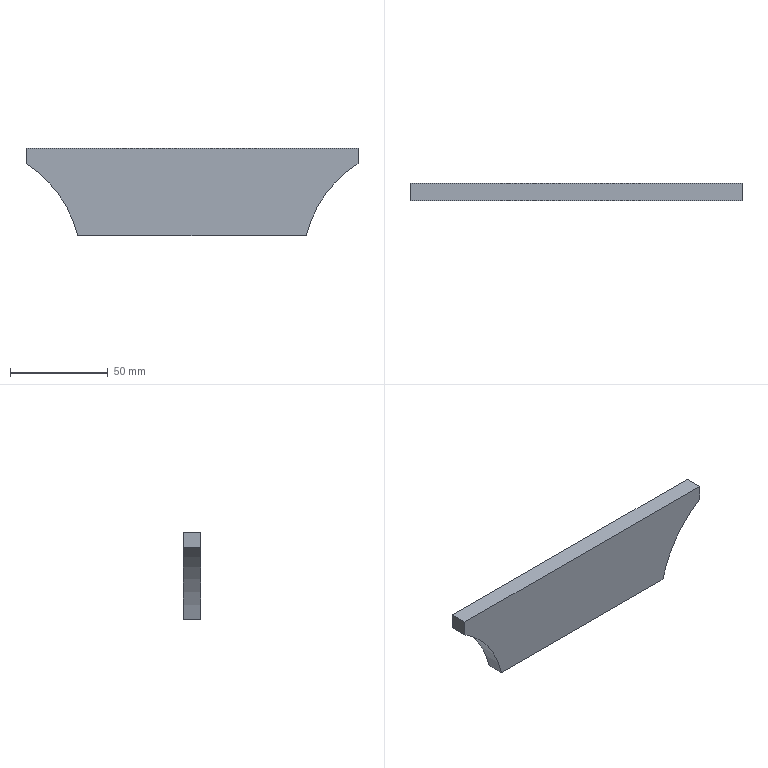Part | SolidWorks | features FlatPattern 1, SMBaseFlange 1, SheetMetal 1 | 1 solid | 8 faces | box 170 x 9 x 45 mm | volume 57559 mm3 | plane 6 | cylinder 2 | commonest cylinder face diameters 120 x2
STEP:
#1=CARTESIAN_POINT('',(0.,0.,-8.));
#2=VERTEX_POINT('',#1);
#3=CARTESIAN_POINT('',(0.,0.,0.));
#4=VERTEX_POINT('',#3);
#5=CARTESIAN_POINT('',(0.,0.,0.));
#6=DIRECTION('',(0.,0.,1.));
#7=VECTOR('',#6,1000.);
#8=LINE('',#5,#7);
#9=EDGE_CURVE('',#2,#4,#8,.T.);
#10=ORIENTED_EDGE('',*,*,#9,.F.);
#11=CARTESIAN_POINT('',(0.,-9.,-8.));
#12=VERTEX_POINT('',#11);
#13=CARTESIAN_POINT('',(0.,-9.,-8.));
#14=DIRECTION('',(0.,1.,0.));
#15=VECTOR('',#14,1000.);
#16=LINE('',#13,#15);
#17=EDGE_CURVE('',#12,#2,#16,.T.);
#18=ORIENTED_EDGE('',*,*,#17,.F.);
#19=CARTESIAN_POINT('',(0.,-9.,0.));
#20=VERTEX_POINT('',#19);
#21=CARTESIAN_POINT('',(0.,-9.,0.));
#22=DIRECTION('',(0.,0.,1.));
#23=VECTOR('',#22,1000.);
#24=LINE('',#21,#23);
#25=EDGE_CURVE('',#12,#20,#24,.T.);
#26=ORIENTED_EDGE('',*,*,#25,.T.);
#27=CARTESIAN_POINT('',(0.,-9.,0.));
#28=DIRECTION('',(0.,1.,0.));
#29=VECTOR('',#28,1000.);
#30=LINE('',#27,#29);
#31=EDGE_CURVE('',#20,#4,#30,.T.);
#32=ORIENTED_EDGE('',*,*,#31,.T.);
#33=EDGE_LOOP('',(#10,#18,#26,#32));
#34=FACE_OUTER_BOUND('',#33,.T.);
#35=CARTESIAN_POINT('',(0.,-9.,0.));
#36=DIRECTION('',(-1.,0.,0.));
#37=DIRECTION('',(0.,0.,1.));
#38=AXIS2_PLACEMENT_3D('',#35,#36,#37);
#39=PLANE('',#38);
#40=ADVANCED_FACE('',(#34),#39,.T.);
#41=CARTESIAN_POINT('',(26.5,0.,-45.));
#42=VERTEX_POINT('',#41);
#43=CARTESIAN_POINT('',(-31.885,0.,-58.827));
#44=DIRECTION('',(0.,-1.,0.));
#45=DIRECTION('',(0.,0.,1.));
#46=AXIS2_PLACEMENT_3D('',#43,#44,#45);
#47=CIRCLE('',#46,60.);
#48=EDGE_CURVE('',#42,#2,#47,.T.);
#49=ORIENTED_EDGE('',*,*,#48,.F.);
#50=CARTESIAN_POINT('',(26.5,-9.,-45.));
#51=VERTEX_POINT('',#50);
#52=CARTESIAN_POINT('',(26.5,-9.,-45.));
#53=DIRECTION('',(0.,1.,0.));
#54=VECTOR('',#53,1000.);
#55=LINE('',#52,#54);
#56=EDGE_CURVE('',#51,#42,#55,.T.);
#57=ORIENTED_EDGE('',*,*,#56,.F.);
#58=CARTESIAN_POINT('',(-31.885,-9.,-58.827));
#59=DIRECTION('',(0.,-1.,0.));
#60=DIRECTION('',(0.,0.,1.));
#61=AXIS2_PLACEMENT_3D('',#58,#59,#60);
#62=CIRCLE('',#61,60.);
#63=EDGE_CURVE('',#51,#12,#62,.T.);
#64=ORIENTED_EDGE('',*,*,#63,.T.);
#65=ORIENTED_EDGE('',*,*,#17,.T.);
#66=EDGE_LOOP('',(#49,#57,#64,#65));
#67=FACE_OUTER_BOUND('',#66,.T.);
#68=CARTESIAN_POINT('',(-31.885,-9.,-58.827));
#69=DIRECTION('',(0.,1.,0.));
#70=DIRECTION('',(0.,0.,1.));
#71=AXIS2_PLACEMENT_3D('',#68,#69,#70);
#72=CYLINDRICAL_SURFACE('',#71,60.);
#73=ADVANCED_FACE('',(#67),#72,.F.);
#74=CARTESIAN_POINT('',(143.5,0.,-45.));
#75=VERTEX_POINT('',#74);
#76=CARTESIAN_POINT('',(26.5,0.,-45.));
#77=DIRECTION('',(-1.,0.,0.));
#78=VECTOR('',#77,1000.);
#79=LINE('',#76,#78);
#80=EDGE_CURVE('',#75,#42,#79,.T.);
#81=ORIENTED_EDGE('',*,*,#80,.F.);
#82=CARTESIAN_POINT('',(143.5,-9.,-45.));
#83=VERTEX_POINT('',#82);
#84=CARTESIAN_POINT('',(143.5,-9.,-45.));
#85=DIRECTION('',(0.,1.,0.));
#86=VECTOR('',#85,1000.);
#87=LINE('',#84,#86);
#88=EDGE_CURVE('',#83,#75,#87,.T.);
#89=ORIENTED_EDGE('',*,*,#88,.F.);
#90=CARTESIAN_POINT('',(26.5,-9.,-45.));
#91=DIRECTION('',(-1.,0.,0.));
#92=VECTOR('',#91,1000.);
#93=LINE('',#90,#92);
#94=EDGE_CURVE('',#83,#51,#93,.T.);
#95=ORIENTED_EDGE('',*,*,#94,.T.);
#96=ORIENTED_EDGE('',*,*,#56,.T.);
#97=EDGE_LOOP('',(#81,#89,#95,#96));
#98=FACE_OUTER_BOUND('',#97,.T.);
#99=CARTESIAN_POINT('',(26.5,-9.,-45.));
#100=DIRECTION('',(0.,0.,-1.));
#101=DIRECTION('',(-1.,0.,0.));
#102=AXIS2_PLACEMENT_3D('',#99,#100,#101);
#103=PLANE('',#102);
#104=ADVANCED_FACE('',(#98),#103,.T.);
#105=CARTESIAN_POINT('',(170.,0.,-8.));
#106=VERTEX_POINT('',#105);
#107=CARTESIAN_POINT('',(201.885,0.,-58.827));
#108=DIRECTION('',(0.,-1.,0.));
#109=DIRECTION('',(0.,0.,-1.));
#110=AXIS2_PLACEMENT_3D('',#107,#108,#109);
#111=CIRCLE('',#110,60.);
#112=EDGE_CURVE('',#106,#75,#111,.T.);
#113=ORIENTED_EDGE('',*,*,#112,.F.);
#114=CARTESIAN_POINT('',(170.,-9.,-8.));
#115=VERTEX_POINT('',#114);
#116=CARTESIAN_POINT('',(170.,-9.,-8.));
#117=DIRECTION('',(0.,1.,0.));
#118=VECTOR('',#117,1000.);
#119=LINE('',#116,#118);
#120=EDGE_CURVE('',#115,#106,#119,.T.);
#121=ORIENTED_EDGE('',*,*,#120,.F.);
#122=CARTESIAN_POINT('',(201.885,-9.,-58.827));
#123=DIRECTION('',(0.,-1.,0.));
#124=DIRECTION('',(0.,0.,-1.));
#125=AXIS2_PLACEMENT_3D('',#122,#123,#124);
#126=CIRCLE('',#125,60.);
#127=EDGE_CURVE('',#115,#83,#126,.T.);
#128=ORIENTED_EDGE('',*,*,#127,.T.);
#129=ORIENTED_EDGE('',*,*,#88,.T.);
#130=EDGE_LOOP('',(#113,#121,#128,#129));
#131=FACE_OUTER_BOUND('',#130,.T.);
#132=CARTESIAN_POINT('',(201.885,-9.,-58.827));
#133=DIRECTION('',(0.,1.,0.));
#134=DIRECTION('',(0.,0.,1.));
#135=AXIS2_PLACEMENT_3D('',#132,#133,#134);
#136=CYLINDRICAL_SURFACE('',#135,60.);
#137=ADVANCED_FACE('',(#131),#136,.F.);
#138=CARTESIAN_POINT('',(170.,0.,0.));
#139=VERTEX_POINT('',#138);
#140=CARTESIAN_POINT('',(170.,0.,0.));
#141=DIRECTION('',(0.,0.,-1.));
#142=VECTOR('',#141,1000.);
#143=LINE('',#140,#142);
#144=EDGE_CURVE('',#139,#106,#143,.T.);
#145=ORIENTED_EDGE('',*,*,#144,.F.);
#146=CARTESIAN_POINT('',(170.,-9.,0.));
#147=VERTEX_POINT('',#146);
#148=CARTESIAN_POINT('',(170.,-9.,0.));
#149=DIRECTION('',(0.,1.,0.));
#150=VECTOR('',#149,1000.);
#151=LINE('',#148,#150);
#152=EDGE_CURVE('',#147,#139,#151,.T.);
#153=ORIENTED_EDGE('',*,*,#152,.F.);
#154=CARTESIAN_POINT('',(170.,-9.,0.));
#155=DIRECTION('',(0.,0.,-1.));
#156=VECTOR('',#155,1000.);
#157=LINE('',#154,#156);
#158=EDGE_CURVE('',#147,#115,#157,.T.);
#159=ORIENTED_EDGE('',*,*,#158,.T.);
#160=ORIENTED_EDGE('',*,*,#120,.T.);
#161=EDGE_LOOP('',(#145,#153,#159,#160));
#162=FACE_OUTER_BOUND('',#161,.T.);
#163=CARTESIAN_POINT('',(170.,-9.,0.));
#164=DIRECTION('',(1.,0.,0.));
#165=DIRECTION('',(0.,0.,-1.));
#166=AXIS2_PLACEMENT_3D('',#163,#164,#165);
#167=PLANE('',#166);
#168=ADVANCED_FACE('',(#162),#167,.T.);
#169=CARTESIAN_POINT('',(0.,0.,0.));
#170=DIRECTION('',(1.,0.,0.));
#171=VECTOR('',#170,1000.);
#172=LINE('',#169,#171);
#173=EDGE_CURVE('',#4,#139,#172,.T.);
#174=ORIENTED_EDGE('',*,*,#173,.F.);
#175=ORIENTED_EDGE('',*,*,#31,.F.);
#176=CARTESIAN_POINT('',(0.,-9.,0.));
#177=DIRECTION('',(1.,0.,0.));
#178=VECTOR('',#177,1000.);
#179=LINE('',#176,#178);
#180=EDGE_CURVE('',#20,#147,#179,.T.);
#181=ORIENTED_EDGE('',*,*,#180,.T.);
#182=ORIENTED_EDGE('',*,*,#152,.T.);
#183=EDGE_LOOP('',(#174,#175,#181,#182));
#184=FACE_OUTER_BOUND('',#183,.T.);
#185=CARTESIAN_POINT('',(0.,-9.,0.));
#186=DIRECTION('',(0.,0.,1.));
#187=DIRECTION('',(1.,0.,0.));
#188=AXIS2_PLACEMENT_3D('',#185,#186,#187);
#189=PLANE('',#188);
#190=ADVANCED_FACE('',(#184),#189,.T.);
#191=ORIENTED_EDGE('',*,*,#25,.F.);
#192=ORIENTED_EDGE('',*,*,#63,.F.);
#193=ORIENTED_EDGE('',*,*,#94,.F.);
#194=ORIENTED_EDGE('',*,*,#127,.F.);
#195=ORIENTED_EDGE('',*,*,#158,.F.);
#196=ORIENTED_EDGE('',*,*,#180,.F.);
#197=EDGE_LOOP('',(#191,#192,#193,#194,#195,#196));
#198=FACE_OUTER_BOUND('',#197,.T.);
#199=CARTESIAN_POINT('',(-31.885,-9.,-58.827));
#200=DIRECTION('',(0.,1.,0.));
#201=DIRECTION('',(0.,0.,1.));
#202=AXIS2_PLACEMENT_3D('',#199,#200,#201);
#203=PLANE('',#202);
#204=ADVANCED_FACE('',(#198),#203,.F.);
#205=ORIENTED_EDGE('',*,*,#9,.T.);
#206=ORIENTED_EDGE('',*,*,#173,.T.);
#207=ORIENTED_EDGE('',*,*,#144,.T.);
#208=ORIENTED_EDGE('',*,*,#112,.T.);
#209=ORIENTED_EDGE('',*,*,#80,.T.);
#210=ORIENTED_EDGE('',*,*,#48,.T.);
#211=EDGE_LOOP('',(#205,#206,#207,#208,#209,#210));
#212=FACE_OUTER_BOUND('',#211,.T.);
#213=CARTESIAN_POINT('',(-31.885,0.,-58.827));
#214=DIRECTION('',(0.,1.,0.));
#215=DIRECTION('',(0.,0.,1.));
#216=AXIS2_PLACEMENT_3D('',#213,#214,#215);
#217=PLANE('',#216);
#218=ADVANCED_FACE('',(#212),#217,.T.);
#219=CLOSED_SHELL('',(#40,#73,#104,#137,#168,#190,#204,#218));
#220=MANIFOLD_SOLID_BREP('',#219);
#221=CARTESIAN_POINT('',(0.,0.,0.));
#222=DIRECTION('',(0.,0.,1.));
#223=DIRECTION('',(1.,0.,0.));
#224=AXIS2_PLACEMENT_3D('',#221,#222,#223);
#225=(LENGTH_UNIT()NAMED_UNIT(*)SI_UNIT(.MILLI.,.METRE.));
#226=UNCERTAINTY_MEASURE_WITH_UNIT(LENGTH_MEASURE(0.00001),#225,'','');
#227=(NAMED_UNIT(*)PLANE_ANGLE_UNIT()SI_UNIT($,.RADIAN.));
#228=(NAMED_UNIT(*)SI_UNIT($,.STERADIAN.)SOLID_ANGLE_UNIT());
#229=(GEOMETRIC_REPRESENTATION_CONTEXT(3)GLOBAL_UNCERTAINTY_ASSIGNED_CONTEXT((#226))GLOBAL_UNIT_ASSIGNED_CONTEXT((#225,#227,#228))REPRESENTATION_CONTEXT('',''));
#230=ADVANCED_BREP_SHAPE_REPRESENTATION('',(#220,#224),#229);